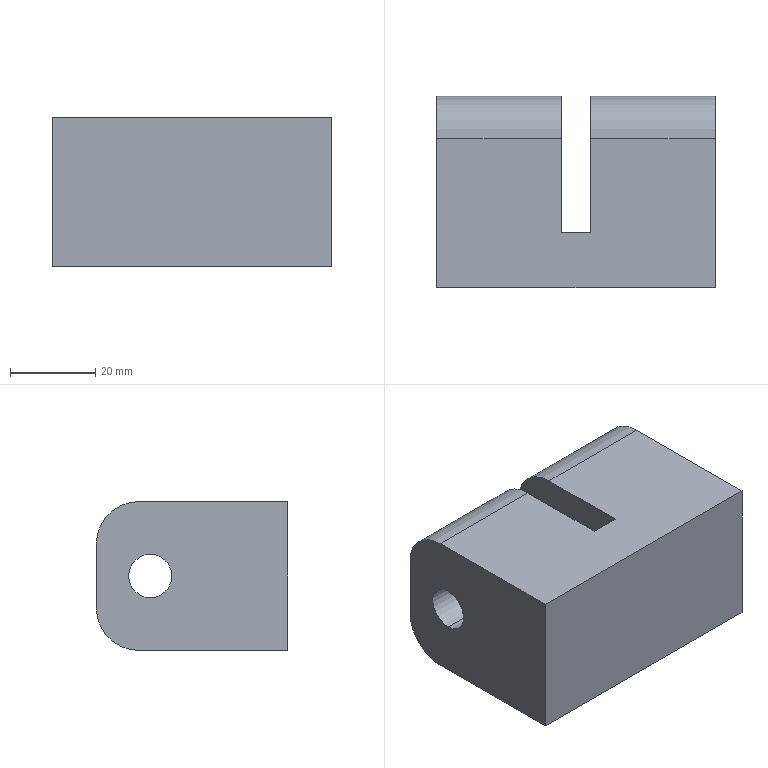Part | SolidWorks | features ICE 2, Extrusion 1, Fillet 1 | 1 solid | 18 faces | box 65.4 x 45 x 35 mm | volume 87886 mm3 | plane 10 | cylinder 8 | commonest cylinder face diameters 10.2 x4 20 x4
STEP:
#1=CARTESIAN_POINT('',(-32.7,9.8,22.6));
#2=VERTEX_POINT('',#1);
#3=CARTESIAN_POINT('',(-32.7,9.8,12.4));
#4=VERTEX_POINT('',#3);
#5=CARTESIAN_POINT('',(-32.7,9.8,17.5));
#6=DIRECTION('',(1.,0.,0.));
#7=DIRECTION('',(0.,1.,0.));
#8=AXIS2_PLACEMENT_3D('',#5,#6,#7);
#9=CIRCLE('',#8,5.1);
#10=EDGE_CURVE('',#2,#4,#9,.T.);
#11=ORIENTED_EDGE('',*,*,#10,.F.);
#12=CARTESIAN_POINT('',(-3.5,9.8,22.6));
#13=VERTEX_POINT('',#12);
#14=CARTESIAN_POINT('',(-51.3,9.8,22.6));
#15=DIRECTION('',(1.,0.,0.));
#16=VECTOR('',#15,1000.);
#17=LINE('',#14,#16);
#18=EDGE_CURVE('',#2,#13,#17,.T.);
#19=ORIENTED_EDGE('',*,*,#18,.T.);
#20=CARTESIAN_POINT('',(-3.5,9.8,12.4));
#21=VERTEX_POINT('',#20);
#22=CARTESIAN_POINT('',(-3.5,9.8,17.5));
#23=DIRECTION('',(1.,0.,0.));
#24=DIRECTION('',(0.,0.,1.));
#25=AXIS2_PLACEMENT_3D('',#22,#23,#24);
#26=CIRCLE('',#25,5.1);
#27=EDGE_CURVE('',#13,#21,#26,.T.);
#28=ORIENTED_EDGE('',*,*,#27,.T.);
#29=CARTESIAN_POINT('',(-51.3,9.8,12.4));
#30=DIRECTION('',(1.,0.,0.));
#31=VECTOR('',#30,1000.);
#32=LINE('',#29,#31);
#33=EDGE_CURVE('',#4,#21,#32,.T.);
#34=ORIENTED_EDGE('',*,*,#33,.F.);
#35=EDGE_LOOP('',(#11,#19,#28,#34));
#36=FACE_OUTER_BOUND('',#35,.T.);
#37=CARTESIAN_POINT('',(-51.3,9.8,17.5));
#38=DIRECTION('',(1.,0.,0.));
#39=DIRECTION('',(0.,0.,-1.));
#40=AXIS2_PLACEMENT_3D('',#37,#38,#39);
#41=CYLINDRICAL_SURFACE('',#40,5.1);
#42=ADVANCED_FACE('',(#36),#41,.F.);
#43=CARTESIAN_POINT('',(3.5,9.8,12.4));
#44=VERTEX_POINT('',#43);
#45=CARTESIAN_POINT('',(3.5,9.8,22.6));
#46=VERTEX_POINT('',#45);
#47=CARTESIAN_POINT('',(3.5,9.8,17.5));
#48=DIRECTION('',(-1.,0.,0.));
#49=DIRECTION('',(0.,0.,-1.));
#50=AXIS2_PLACEMENT_3D('',#47,#48,#49);
#51=CIRCLE('',#50,5.1);
#52=EDGE_CURVE('',#44,#46,#51,.T.);
#53=ORIENTED_EDGE('',*,*,#52,.T.);
#54=CARTESIAN_POINT('',(32.7,9.8,22.6));
#55=VERTEX_POINT('',#54);
#56=CARTESIAN_POINT('',(-51.3,9.8,22.6));
#57=DIRECTION('',(1.,0.,0.));
#58=VECTOR('',#57,1000.);
#59=LINE('',#56,#58);
#60=EDGE_CURVE('',#46,#55,#59,.T.);
#61=ORIENTED_EDGE('',*,*,#60,.T.);
#62=CARTESIAN_POINT('',(32.7,9.8,12.4));
#63=VERTEX_POINT('',#62);
#64=CARTESIAN_POINT('',(32.7,9.8,17.5));
#65=DIRECTION('',(1.,0.,0.));
#66=DIRECTION('',(0.,0.,-1.));
#67=AXIS2_PLACEMENT_3D('',#64,#65,#66);
#68=CIRCLE('',#67,5.1);
#69=EDGE_CURVE('',#55,#63,#68,.T.);
#70=ORIENTED_EDGE('',*,*,#69,.T.);
#71=CARTESIAN_POINT('',(-51.3,9.8,12.4));
#72=DIRECTION('',(1.,0.,0.));
#73=VECTOR('',#72,1000.);
#74=LINE('',#71,#73);
#75=EDGE_CURVE('',#44,#63,#74,.T.);
#76=ORIENTED_EDGE('',*,*,#75,.F.);
#77=EDGE_LOOP('',(#53,#61,#70,#76));
#78=FACE_OUTER_BOUND('',#77,.T.);
#79=CARTESIAN_POINT('',(-51.3,9.8,17.5));
#80=DIRECTION('',(1.,0.,0.));
#81=DIRECTION('',(0.,0.,-1.));
#82=AXIS2_PLACEMENT_3D('',#79,#80,#81);
#83=CYLINDRICAL_SURFACE('',#82,5.1);
#84=ADVANCED_FACE('',(#78),#83,.F.);
#85=CARTESIAN_POINT('',(32.7,22.5,10.));
#86=VERTEX_POINT('',#85);
#87=CARTESIAN_POINT('',(3.5,22.5,10.));
#88=VERTEX_POINT('',#87);
#89=CARTESIAN_POINT('',(-32.7,22.5,10.));
#90=DIRECTION('',(-1.,0.,0.));
#91=VECTOR('',#90,1000.);
#92=LINE('',#89,#91);
#93=EDGE_CURVE('',#86,#88,#92,.T.);
#94=ORIENTED_EDGE('',*,*,#93,.T.);
#95=CARTESIAN_POINT('',(3.5,22.5,25.));
#96=VERTEX_POINT('',#95);
#97=CARTESIAN_POINT('',(3.5,22.5,35.));
#98=DIRECTION('',(0.,0.,1.));
#99=VECTOR('',#98,1000.);
#100=LINE('',#97,#99);
#101=EDGE_CURVE('',#88,#96,#100,.T.);
#102=ORIENTED_EDGE('',*,*,#101,.T.);
#103=CARTESIAN_POINT('',(32.7,22.5,25.));
#104=VERTEX_POINT('',#103);
#105=CARTESIAN_POINT('',(32.7,22.5,25.));
#106=DIRECTION('',(1.,0.,0.));
#107=VECTOR('',#106,1000.);
#108=LINE('',#105,#107);
#109=EDGE_CURVE('',#96,#104,#108,.T.);
#110=ORIENTED_EDGE('',*,*,#109,.T.);
#111=CARTESIAN_POINT('',(32.7,22.5,35.));
#112=DIRECTION('',(0.,0.,-1.));
#113=VECTOR('',#112,1000.);
#114=LINE('',#111,#113);
#115=EDGE_CURVE('',#104,#86,#114,.T.);
#116=ORIENTED_EDGE('',*,*,#115,.T.);
#117=EDGE_LOOP('',(#94,#102,#110,#116));
#118=FACE_OUTER_BOUND('',#117,.T.);
#119=CARTESIAN_POINT('',(32.7,22.5,35.));
#120=DIRECTION('',(0.,-1.,0.));
#121=DIRECTION('',(1.,0.,0.));
#122=AXIS2_PLACEMENT_3D('',#119,#120,#121);
#123=PLANE('',#122);
#124=ADVANCED_FACE('',(#118),#123,.F.);
#125=CARTESIAN_POINT('',(3.5,12.5,0.));
#126=VERTEX_POINT('',#125);
#127=CARTESIAN_POINT('',(3.5,12.5,10.));
#128=DIRECTION('',(-1.,0.,0.));
#129=DIRECTION('',(0.,0.,-1.));
#130=AXIS2_PLACEMENT_3D('',#127,#128,#129);
#131=CIRCLE('',#130,10.);
#132=EDGE_CURVE('',#88,#126,#131,.T.);
#133=ORIENTED_EDGE('',*,*,#132,.F.);
#134=ORIENTED_EDGE('',*,*,#93,.F.);
#135=CARTESIAN_POINT('',(32.7,12.5,0.));
#136=VERTEX_POINT('',#135);
#137=CARTESIAN_POINT('',(32.7,12.5,10.));
#138=DIRECTION('',(1.,0.,0.));
#139=DIRECTION('',(0.,0.,1.));
#140=AXIS2_PLACEMENT_3D('',#137,#138,#139);
#141=CIRCLE('',#140,10.);
#142=EDGE_CURVE('',#136,#86,#141,.T.);
#143=ORIENTED_EDGE('',*,*,#142,.F.);
#144=CARTESIAN_POINT('',(32.7,12.5,0.));
#145=DIRECTION('',(1.,0.,0.));
#146=VECTOR('',#145,1000.);
#147=LINE('',#144,#146);
#148=EDGE_CURVE('',#126,#136,#147,.T.);
#149=ORIENTED_EDGE('',*,*,#148,.F.);
#150=EDGE_LOOP('',(#133,#134,#143,#149));
#151=FACE_OUTER_BOUND('',#150,.T.);
#152=CARTESIAN_POINT('',(32.7,12.5,10.));
#153=DIRECTION('',(1.,0.,0.));
#154=DIRECTION('',(0.,1.,0.));
#155=AXIS2_PLACEMENT_3D('',#152,#153,#154);
#156=CYLINDRICAL_SURFACE('',#155,10.);
#157=ADVANCED_FACE('',(#151),#156,.T.);
#158=CARTESIAN_POINT('',(3.5,12.5,35.));
#159=VERTEX_POINT('',#158);
#160=CARTESIAN_POINT('',(3.5,12.5,25.));
#161=DIRECTION('',(-1.,0.,0.));
#162=DIRECTION('',(0.,0.,-1.));
#163=AXIS2_PLACEMENT_3D('',#160,#161,#162);
#164=CIRCLE('',#163,10.);
#165=EDGE_CURVE('',#159,#96,#164,.T.);
#166=ORIENTED_EDGE('',*,*,#165,.F.);
#167=CARTESIAN_POINT('',(32.7,12.5,35.));
#168=VERTEX_POINT('',#167);
#169=CARTESIAN_POINT('',(0.,12.5,35.));
#170=DIRECTION('',(-1.,0.,0.));
#171=VECTOR('',#170,1000.);
#172=LINE('',#169,#171);
#173=EDGE_CURVE('',#168,#159,#172,.T.);
#174=ORIENTED_EDGE('',*,*,#173,.F.);
#175=CARTESIAN_POINT('',(32.7,12.5,25.));
#176=DIRECTION('',(1.,0.,0.));
#177=DIRECTION('',(0.,0.,1.));
#178=AXIS2_PLACEMENT_3D('',#175,#176,#177);
#179=CIRCLE('',#178,10.);
#180=EDGE_CURVE('',#104,#168,#179,.T.);
#181=ORIENTED_EDGE('',*,*,#180,.F.);
#182=ORIENTED_EDGE('',*,*,#109,.F.);
#183=EDGE_LOOP('',(#166,#174,#181,#182));
#184=FACE_OUTER_BOUND('',#183,.T.);
#185=CARTESIAN_POINT('',(0.,12.5,25.));
#186=DIRECTION('',(-1.,0.,0.));
#187=DIRECTION('',(0.,-1.,0.));
#188=AXIS2_PLACEMENT_3D('',#185,#186,#187);
#189=CYLINDRICAL_SURFACE('',#188,10.);
#190=ADVANCED_FACE('',(#184),#189,.T.);
#191=ORIENTED_EDGE('',*,*,#60,.F.);
#192=CARTESIAN_POINT('',(3.5,9.8,17.5));
#193=DIRECTION('',(-1.,0.,0.));
#194=DIRECTION('',(0.,0.,-1.));
#195=AXIS2_PLACEMENT_3D('',#192,#193,#194);
#196=CIRCLE('',#195,5.1);
#197=EDGE_CURVE('',#46,#44,#196,.T.);
#198=ORIENTED_EDGE('',*,*,#197,.T.);
#199=ORIENTED_EDGE('',*,*,#75,.T.);
#200=CARTESIAN_POINT('',(32.7,9.8,17.5));
#201=DIRECTION('',(1.,0.,0.));
#202=DIRECTION('',(0.,0.,-1.));
#203=AXIS2_PLACEMENT_3D('',#200,#201,#202);
#204=CIRCLE('',#203,5.1);
#205=EDGE_CURVE('',#63,#55,#204,.T.);
#206=ORIENTED_EDGE('',*,*,#205,.T.);
#207=EDGE_LOOP('',(#191,#198,#199,#206));
#208=FACE_OUTER_BOUND('',#207,.T.);
#209=CARTESIAN_POINT('',(-51.3,9.8,17.5));
#210=DIRECTION('',(1.,0.,0.));
#211=DIRECTION('',(0.,0.,-1.));
#212=AXIS2_PLACEMENT_3D('',#209,#210,#211);
#213=CYLINDRICAL_SURFACE('',#212,5.1);
#214=ADVANCED_FACE('',(#208),#213,.F.);
#215=CARTESIAN_POINT('',(-32.7,9.8,17.5));
#216=DIRECTION('',(1.,0.,0.));
#217=DIRECTION('',(0.,1.,0.));
#218=AXIS2_PLACEMENT_3D('',#215,#216,#217);
#219=CIRCLE('',#218,5.1);
#220=EDGE_CURVE('',#4,#2,#219,.T.);
#221=ORIENTED_EDGE('',*,*,#220,.T.);
#222=ORIENTED_EDGE('',*,*,#10,.T.);
#223=EDGE_LOOP('',(#221,#222));
#224=FACE_BOUND('',#223,.T.);
#225=CARTESIAN_POINT('',(-32.7,22.5,25.));
#226=VERTEX_POINT('',#225);
#227=CARTESIAN_POINT('',(-32.7,22.5,10.));
#228=VERTEX_POINT('',#227);
#229=CARTESIAN_POINT('',(-32.7,22.5,35.));
#230=DIRECTION('',(0.,0.,-1.));
#231=VECTOR('',#230,1000.);
#232=LINE('',#229,#231);
#233=EDGE_CURVE('',#226,#228,#232,.T.);
#234=ORIENTED_EDGE('',*,*,#233,.T.);
#235=CARTESIAN_POINT('',(-32.7,12.5,0.));
#236=VERTEX_POINT('',#235);
#237=CARTESIAN_POINT('',(-32.7,12.5,10.));
#238=DIRECTION('',(-1.,0.,0.));
#239=DIRECTION('',(0.,1.,0.));
#240=AXIS2_PLACEMENT_3D('',#237,#238,#239);
#241=CIRCLE('',#240,10.);
#242=EDGE_CURVE('',#228,#236,#241,.T.);
#243=ORIENTED_EDGE('',*,*,#242,.T.);
#244=CARTESIAN_POINT('',(-32.7,-22.5,0.));
#245=VERTEX_POINT('',#244);
#246=CARTESIAN_POINT('',(-32.7,22.5,0.));
#247=DIRECTION('',(0.,-1.,0.));
#248=VECTOR('',#247,1000.);
#249=LINE('',#246,#248);
#250=EDGE_CURVE('',#236,#245,#249,.T.);
#251=ORIENTED_EDGE('',*,*,#250,.T.);
#252=CARTESIAN_POINT('',(-32.7,-22.5,35.));
#253=VERTEX_POINT('',#252);
#254=CARTESIAN_POINT('',(-32.7,-22.5,35.));
#255=DIRECTION('',(0.,0.,-1.));
#256=VECTOR('',#255,1000.);
#257=LINE('',#254,#256);
#258=EDGE_CURVE('',#253,#245,#257,.T.);
#259=ORIENTED_EDGE('',*,*,#258,.F.);
#260=CARTESIAN_POINT('',(-32.7,12.5,35.));
#261=VERTEX_POINT('',#260);
#262=CARTESIAN_POINT('',(-32.7,22.5,35.));
#263=DIRECTION('',(0.,-1.,0.));
#264=VECTOR('',#263,1000.);
#265=LINE('',#262,#264);
#266=EDGE_CURVE('',#261,#253,#265,.T.);
#267=ORIENTED_EDGE('',*,*,#266,.F.);
#268=CARTESIAN_POINT('',(-32.7,12.5,25.));
#269=DIRECTION('',(-1.,0.,0.));
#270=DIRECTION('',(0.,1.,0.));
#271=AXIS2_PLACEMENT_3D('',#268,#269,#270);
#272=CIRCLE('',#271,10.);
#273=EDGE_CURVE('',#261,#226,#272,.T.);
#274=ORIENTED_EDGE('',*,*,#273,.T.);
#275=EDGE_LOOP('',(#234,#243,#251,#259,#267,#274));
#276=FACE_OUTER_BOUND('',#275,.T.);
#277=CARTESIAN_POINT('',(-32.7,22.5,35.));
#278=DIRECTION('',(1.,0.,0.));
#279=DIRECTION('',(0.,1.,0.));
#280=AXIS2_PLACEMENT_3D('',#277,#278,#279);
#281=PLANE('',#280);
#282=ADVANCED_FACE('',(#224,#276),#281,.F.);
#283=CARTESIAN_POINT('',(32.7,-22.5,0.));
#284=VERTEX_POINT('',#283);
#285=CARTESIAN_POINT('',(32.7,-22.5,0.));
#286=DIRECTION('',(1.,0.,0.));
#287=VECTOR('',#286,1000.);
#288=LINE('',#285,#287);
#289=EDGE_CURVE('',#245,#284,#288,.T.);
#290=ORIENTED_EDGE('',*,*,#289,.T.);
#291=CARTESIAN_POINT('',(32.7,-22.5,35.));
#292=VERTEX_POINT('',#291);
#293=CARTESIAN_POINT('',(32.7,-22.5,35.));
#294=DIRECTION('',(0.,0.,-1.));
#295=VECTOR('',#294,1000.);
#296=LINE('',#293,#295);
#297=EDGE_CURVE('',#292,#284,#296,.T.);
#298=ORIENTED_EDGE('',*,*,#297,.F.);
#299=CARTESIAN_POINT('',(32.7,-22.5,35.));
#300=DIRECTION('',(1.,0.,0.));
#301=VECTOR('',#300,1000.);
#302=LINE('',#299,#301);
#303=EDGE_CURVE('',#253,#292,#302,.T.);
#304=ORIENTED_EDGE('',*,*,#303,.F.);
#305=ORIENTED_EDGE('',*,*,#258,.T.);
#306=EDGE_LOOP('',(#290,#298,#304,#305));
#307=FACE_OUTER_BOUND('',#306,.T.);
#308=CARTESIAN_POINT('',(32.7,-22.5,35.));
#309=DIRECTION('',(0.,1.,0.));
#310=DIRECTION('',(-1.,0.,0.));
#311=AXIS2_PLACEMENT_3D('',#308,#309,#310);
#312=PLANE('',#311);
#313=ADVANCED_FACE('',(#307),#312,.F.);
#314=ORIENTED_EDGE('',*,*,#205,.F.);
#315=ORIENTED_EDGE('',*,*,#69,.F.);
#316=EDGE_LOOP('',(#314,#315));
#317=FACE_BOUND('',#316,.T.);
#318=CARTESIAN_POINT('',(32.7,22.5,0.));
#319=DIRECTION('',(0.,1.,0.));
#320=VECTOR('',#319,1000.);
#321=LINE('',#318,#320);
#322=EDGE_CURVE('',#284,#136,#321,.T.);
#323=ORIENTED_EDGE('',*,*,#322,.T.);
#324=ORIENTED_EDGE('',*,*,#142,.T.);
#325=ORIENTED_EDGE('',*,*,#115,.F.);
#326=ORIENTED_EDGE('',*,*,#180,.T.);
#327=CARTESIAN_POINT('',(32.7,22.5,35.));
#328=DIRECTION('',(0.,1.,0.));
#329=VECTOR('',#328,1000.);
#330=LINE('',#327,#329);
#331=EDGE_CURVE('',#292,#168,#330,.T.);
#332=ORIENTED_EDGE('',*,*,#331,.F.);
#333=ORIENTED_EDGE('',*,*,#297,.T.);
#334=EDGE_LOOP('',(#323,#324,#325,#326,#332,#333));
#335=FACE_OUTER_BOUND('',#334,.T.);
#336=CARTESIAN_POINT('',(32.7,22.5,35.));
#337=DIRECTION('',(-1.,0.,0.));
#338=DIRECTION('',(0.,0.,1.));
#339=AXIS2_PLACEMENT_3D('',#336,#337,#338);
#340=PLANE('',#339);
#341=ADVANCED_FACE('',(#317,#335),#340,.F.);
#342=CARTESIAN_POINT('',(-3.5,22.5,25.));
#343=VERTEX_POINT('',#342);
#344=CARTESIAN_POINT('',(32.7,22.5,25.));
#345=DIRECTION('',(1.,0.,0.));
#346=VECTOR('',#345,1000.);
#347=LINE('',#344,#346);
#348=EDGE_CURVE('',#226,#343,#347,.T.);
#349=ORIENTED_EDGE('',*,*,#348,.T.);
#350=CARTESIAN_POINT('',(-3.5,22.5,10.));
#351=VERTEX_POINT('',#350);
#352=CARTESIAN_POINT('',(-3.5,22.5,35.));
#353=DIRECTION('',(0.,0.,-1.));
#354=VECTOR('',#353,1000.);
#355=LINE('',#352,#354);
#356=EDGE_CURVE('',#343,#351,#355,.T.);
#357=ORIENTED_EDGE('',*,*,#356,.T.);
#358=CARTESIAN_POINT('',(-32.7,22.5,10.));
#359=DIRECTION('',(-1.,0.,0.));
#360=VECTOR('',#359,1000.);
#361=LINE('',#358,#360);
#362=EDGE_CURVE('',#351,#228,#361,.T.);
#363=ORIENTED_EDGE('',*,*,#362,.T.);
#364=ORIENTED_EDGE('',*,*,#233,.F.);
#365=EDGE_LOOP('',(#349,#357,#363,#364));
#366=FACE_OUTER_BOUND('',#365,.T.);
#367=CARTESIAN_POINT('',(32.7,22.5,35.));
#368=DIRECTION('',(0.,-1.,0.));
#369=DIRECTION('',(1.,0.,0.));
#370=AXIS2_PLACEMENT_3D('',#367,#368,#369);
#371=PLANE('',#370);
#372=ADVANCED_FACE('',(#366),#371,.F.);
#373=ORIENTED_EDGE('',*,*,#173,.T.);
#374=CARTESIAN_POINT('',(3.5,-9.5,35.));
#375=VERTEX_POINT('',#374);
#376=CARTESIAN_POINT('',(3.5,-9.5,35.));
#377=DIRECTION('',(0.,1.,0.));
#378=VECTOR('',#377,1000.);
#379=LINE('',#376,#378);
#380=EDGE_CURVE('',#375,#159,#379,.T.);
#381=ORIENTED_EDGE('',*,*,#380,.F.);
#382=CARTESIAN_POINT('',(-3.5,-9.5,35.));
#383=VERTEX_POINT('',#382);
#384=CARTESIAN_POINT('',(3.5,-9.5,35.));
#385=DIRECTION('',(1.,0.,0.));
#386=VECTOR('',#385,1000.);
#387=LINE('',#384,#386);
#388=EDGE_CURVE('',#383,#375,#387,.T.);
#389=ORIENTED_EDGE('',*,*,#388,.F.);
#390=CARTESIAN_POINT('',(-3.5,12.5,35.));
#391=VERTEX_POINT('',#390);
#392=CARTESIAN_POINT('',(-3.5,-9.5,35.));
#393=DIRECTION('',(0.,-1.,0.));
#394=VECTOR('',#393,1000.);
#395=LINE('',#392,#394);
#396=EDGE_CURVE('',#391,#383,#395,.T.);
#397=ORIENTED_EDGE('',*,*,#396,.F.);
#398=CARTESIAN_POINT('',(0.,12.5,35.));
#399=DIRECTION('',(-1.,0.,0.));
#400=VECTOR('',#399,1000.);
#401=LINE('',#398,#400);
#402=EDGE_CURVE('',#391,#261,#401,.T.);
#403=ORIENTED_EDGE('',*,*,#402,.T.);
#404=ORIENTED_EDGE('',*,*,#266,.T.);
#405=ORIENTED_EDGE('',*,*,#303,.T.);
#406=ORIENTED_EDGE('',*,*,#331,.T.);
#407=EDGE_LOOP('',(#373,#381,#389,#397,#403,#404,#405,#406));
#408=FACE_OUTER_BOUND('',#407,.T.);
#409=CARTESIAN_POINT('',(0.,0.,35.));
#410=DIRECTION('',(0.,0.,-1.));
#411=DIRECTION('',(-1.,0.,0.));
#412=AXIS2_PLACEMENT_3D('',#409,#410,#411);
#413=PLANE('',#412);
#414=ADVANCED_FACE('',(#408),#413,.F.);
#415=CARTESIAN_POINT('',(3.5,-9.5,0.));
#416=VERTEX_POINT('',#415);
#417=CARTESIAN_POINT('',(3.5,-9.5,0.));
#418=DIRECTION('',(0.,1.,0.));
#419=VECTOR('',#418,1000.);
#420=LINE('',#417,#419);
#421=EDGE_CURVE('',#416,#126,#420,.T.);
#422=ORIENTED_EDGE('',*,*,#421,.T.);
#423=ORIENTED_EDGE('',*,*,#148,.T.);
#424=ORIENTED_EDGE('',*,*,#322,.F.);
#425=ORIENTED_EDGE('',*,*,#289,.F.);
#426=ORIENTED_EDGE('',*,*,#250,.F.);
#427=CARTESIAN_POINT('',(-3.5,12.5,0.));
#428=VERTEX_POINT('',#427);
#429=CARTESIAN_POINT('',(32.7,12.5,0.));
#430=DIRECTION('',(1.,0.,0.));
#431=VECTOR('',#430,1000.);
#432=LINE('',#429,#431);
#433=EDGE_CURVE('',#236,#428,#432,.T.);
#434=ORIENTED_EDGE('',*,*,#433,.T.);
#435=CARTESIAN_POINT('',(-3.5,-9.5,0.));
#436=VERTEX_POINT('',#435);
#437=CARTESIAN_POINT('',(-3.5,-9.5,0.));
#438=DIRECTION('',(0.,-1.,0.));
#439=VECTOR('',#438,1000.);
#440=LINE('',#437,#439);
#441=EDGE_CURVE('',#428,#436,#440,.T.);
#442=ORIENTED_EDGE('',*,*,#441,.T.);
#443=CARTESIAN_POINT('',(3.5,-9.5,0.));
#444=DIRECTION('',(1.,0.,0.));
#445=VECTOR('',#444,1000.);
#446=LINE('',#443,#445);
#447=EDGE_CURVE('',#436,#416,#446,.T.);
#448=ORIENTED_EDGE('',*,*,#447,.T.);
#449=EDGE_LOOP('',(#422,#423,#424,#425,#426,#434,#442,#448));
#450=FACE_OUTER_BOUND('',#449,.T.);
#451=CARTESIAN_POINT('',(0.,0.,0.));
#452=DIRECTION('',(0.,0.,-1.));
#453=DIRECTION('',(-1.,0.,0.));
#454=AXIS2_PLACEMENT_3D('',#451,#452,#453);
#455=PLANE('',#454);
#456=ADVANCED_FACE('',(#450),#455,.T.);
#457=CARTESIAN_POINT('',(-3.5,12.5,10.));
#458=DIRECTION('',(1.,0.,0.));
#459=DIRECTION('',(0.,0.,1.));
#460=AXIS2_PLACEMENT_3D('',#457,#458,#459);
#461=CIRCLE('',#460,10.);
#462=EDGE_CURVE('',#428,#351,#461,.T.);
#463=ORIENTED_EDGE('',*,*,#462,.F.);
#464=ORIENTED_EDGE('',*,*,#433,.F.);
#465=ORIENTED_EDGE('',*,*,#242,.F.);
#466=ORIENTED_EDGE('',*,*,#362,.F.);
#467=EDGE_LOOP('',(#463,#464,#465,#466));
#468=FACE_OUTER_BOUND('',#467,.T.);
#469=CARTESIAN_POINT('',(32.7,12.5,10.));
#470=DIRECTION('',(1.,0.,0.));
#471=DIRECTION('',(0.,1.,0.));
#472=AXIS2_PLACEMENT_3D('',#469,#470,#471);
#473=CYLINDRICAL_SURFACE('',#472,10.);
#474=ADVANCED_FACE('',(#468),#473,.T.);
#475=CARTESIAN_POINT('',(-3.5,12.5,25.));
#476=DIRECTION('',(1.,0.,0.));
#477=DIRECTION('',(0.,0.,1.));
#478=AXIS2_PLACEMENT_3D('',#475,#476,#477);
#479=CIRCLE('',#478,10.);
#480=EDGE_CURVE('',#343,#391,#479,.T.);
#481=ORIENTED_EDGE('',*,*,#480,.F.);
#482=ORIENTED_EDGE('',*,*,#348,.F.);
#483=ORIENTED_EDGE('',*,*,#273,.F.);
#484=ORIENTED_EDGE('',*,*,#402,.F.);
#485=EDGE_LOOP('',(#481,#482,#483,#484));
#486=FACE_OUTER_BOUND('',#485,.T.);
#487=CARTESIAN_POINT('',(0.,12.5,25.));
#488=DIRECTION('',(-1.,0.,0.));
#489=DIRECTION('',(0.,-1.,0.));
#490=AXIS2_PLACEMENT_3D('',#487,#488,#489);
#491=CYLINDRICAL_SURFACE('',#490,10.);
#492=ADVANCED_FACE('',(#486),#491,.T.);
#493=ORIENTED_EDGE('',*,*,#18,.F.);
#494=ORIENTED_EDGE('',*,*,#220,.F.);
#495=ORIENTED_EDGE('',*,*,#33,.T.);
#496=CARTESIAN_POINT('',(-3.5,9.8,17.5));
#497=DIRECTION('',(1.,0.,0.));
#498=DIRECTION('',(0.,0.,1.));
#499=AXIS2_PLACEMENT_3D('',#496,#497,#498);
#500=CIRCLE('',#499,5.1);
#501=EDGE_CURVE('',#21,#13,#500,.T.);
#502=ORIENTED_EDGE('',*,*,#501,.T.);
#503=EDGE_LOOP('',(#493,#494,#495,#502));
#504=FACE_OUTER_BOUND('',#503,.T.);
#505=CARTESIAN_POINT('',(-51.3,9.8,17.5));
#506=DIRECTION('',(1.,0.,0.));
#507=DIRECTION('',(0.,0.,-1.));
#508=AXIS2_PLACEMENT_3D('',#505,#506,#507);
#509=CYLINDRICAL_SURFACE('',#508,5.1);
#510=ADVANCED_FACE('',(#504),#509,.F.);
#511=ORIENTED_EDGE('',*,*,#132,.T.);
#512=ORIENTED_EDGE('',*,*,#421,.F.);
#513=CARTESIAN_POINT('',(3.5,-9.5,0.));
#514=DIRECTION('',(0.,0.,1.));
#515=VECTOR('',#514,1000.);
#516=LINE('',#513,#515);
#517=EDGE_CURVE('',#416,#375,#516,.T.);
#518=ORIENTED_EDGE('',*,*,#517,.T.);
#519=ORIENTED_EDGE('',*,*,#380,.T.);
#520=ORIENTED_EDGE('',*,*,#165,.T.);
#521=ORIENTED_EDGE('',*,*,#101,.F.);
#522=EDGE_LOOP('',(#511,#512,#518,#519,#520,#521));
#523=FACE_OUTER_BOUND('',#522,.T.);
#524=ORIENTED_EDGE('',*,*,#52,.F.);
#525=ORIENTED_EDGE('',*,*,#197,.F.);
#526=EDGE_LOOP('',(#524,#525));
#527=FACE_BOUND('',#526,.T.);
#528=CARTESIAN_POINT('',(3.5,-9.5,0.));
#529=DIRECTION('',(1.,0.,0.));
#530=DIRECTION('',(0.,0.,-1.));
#531=AXIS2_PLACEMENT_3D('',#528,#529,#530);
#532=PLANE('',#531);
#533=ADVANCED_FACE('',(#523,#527),#532,.F.);
#534=ORIENTED_EDGE('',*,*,#462,.T.);
#535=ORIENTED_EDGE('',*,*,#356,.F.);
#536=ORIENTED_EDGE('',*,*,#480,.T.);
#537=ORIENTED_EDGE('',*,*,#396,.T.);
#538=CARTESIAN_POINT('',(-3.5,-9.5,0.));
#539=DIRECTION('',(0.,0.,1.));
#540=VECTOR('',#539,1000.);
#541=LINE('',#538,#540);
#542=EDGE_CURVE('',#436,#383,#541,.T.);
#543=ORIENTED_EDGE('',*,*,#542,.F.);
#544=ORIENTED_EDGE('',*,*,#441,.F.);
#545=EDGE_LOOP('',(#534,#535,#536,#537,#543,#544));
#546=FACE_OUTER_BOUND('',#545,.T.);
#547=ORIENTED_EDGE('',*,*,#501,.F.);
#548=ORIENTED_EDGE('',*,*,#27,.F.);
#549=EDGE_LOOP('',(#547,#548));
#550=FACE_BOUND('',#549,.T.);
#551=CARTESIAN_POINT('',(-3.5,-9.5,0.));
#552=DIRECTION('',(-1.,0.,0.));
#553=DIRECTION('',(0.,0.,1.));
#554=AXIS2_PLACEMENT_3D('',#551,#552,#553);
#555=PLANE('',#554);
#556=ADVANCED_FACE('',(#546,#550),#555,.F.);
#557=ORIENTED_EDGE('',*,*,#388,.T.);
#558=ORIENTED_EDGE('',*,*,#517,.F.);
#559=ORIENTED_EDGE('',*,*,#447,.F.);
#560=ORIENTED_EDGE('',*,*,#542,.T.);
#561=EDGE_LOOP('',(#557,#558,#559,#560));
#562=FACE_OUTER_BOUND('',#561,.T.);
#563=CARTESIAN_POINT('',(3.5,-9.5,0.));
#564=DIRECTION('',(0.,-1.,0.));
#565=DIRECTION('',(0.,0.,-1.));
#566=AXIS2_PLACEMENT_3D('',#563,#564,#565);
#567=PLANE('',#566);
#568=ADVANCED_FACE('',(#562),#567,.F.);
#569=CLOSED_SHELL('',(#42,#84,#124,#157,#190,#214,#282,#313,#341,#372,#414,#456,#474,#492,#510,#533,#556,#568));
#570=MANIFOLD_SOLID_BREP('',#569);
#571=CARTESIAN_POINT('',(0.,0.,0.));
#572=DIRECTION('',(0.,0.,1.));
#573=DIRECTION('',(1.,0.,0.));
#574=AXIS2_PLACEMENT_3D('',#571,#572,#573);
#575=(LENGTH_UNIT()NAMED_UNIT(*)SI_UNIT(.MILLI.,.METRE.));
#576=UNCERTAINTY_MEASURE_WITH_UNIT(LENGTH_MEASURE(0.00001),#575,'','');
#577=(NAMED_UNIT(*)PLANE_ANGLE_UNIT()SI_UNIT($,.RADIAN.));
#578=(NAMED_UNIT(*)SI_UNIT($,.STERADIAN.)SOLID_ANGLE_UNIT());
#579=(GEOMETRIC_REPRESENTATION_CONTEXT(3)GLOBAL_UNCERTAINTY_ASSIGNED_CONTEXT((#576))GLOBAL_UNIT_ASSIGNED_CONTEXT((#575,#577,#578))REPRESENTATION_CONTEXT('',''));
#580=ADVANCED_BREP_SHAPE_REPRESENTATION('',(#570,#574),#579);